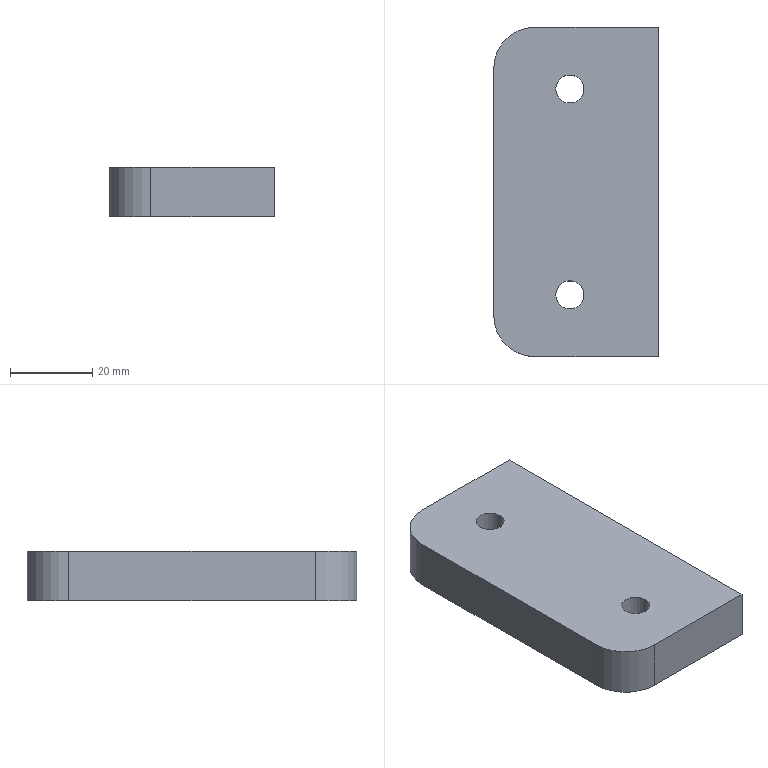Part | SolidWorks | features BaseBody 1 | 1 solid | 12 faces | box 40 x 80 x 12 mm | volume 37013 mm3 | cylinder 6 | plane 6 | commonest cylinder face diameters 6.8 x4 20 x2
STEP:
#1=CARTESIAN_POINT('',(-4.9,25.,0.));
#2=VERTEX_POINT('',#1);
#3=CARTESIAN_POINT('',(1.9,25.,0.));
#4=VERTEX_POINT('',#3);
#5=CARTESIAN_POINT('',(-1.5,25.,0.));
#6=DIRECTION('',(0.,0.,1.));
#7=DIRECTION('',(1.,0.,0.));
#8=AXIS2_PLACEMENT_3D('',#5,#6,#7);
#9=CIRCLE('',#8,3.4);
#10=EDGE_CURVE('',#2,#4,#9,.T.);
#11=ORIENTED_EDGE('',*,*,#10,.F.);
#12=CARTESIAN_POINT('',(-4.9,25.,12.));
#13=VERTEX_POINT('',#12);
#14=CARTESIAN_POINT('',(-4.9,25.,12.));
#15=DIRECTION('',(0.,0.,1.));
#16=VECTOR('',#15,1000.);
#17=LINE('',#14,#16);
#18=EDGE_CURVE('',#2,#13,#17,.T.);
#19=ORIENTED_EDGE('',*,*,#18,.T.);
#20=CARTESIAN_POINT('',(1.9,25.,12.));
#21=VERTEX_POINT('',#20);
#22=CARTESIAN_POINT('',(-1.5,25.,12.));
#23=DIRECTION('',(0.,0.,1.));
#24=DIRECTION('',(1.,0.,0.));
#25=AXIS2_PLACEMENT_3D('',#22,#23,#24);
#26=CIRCLE('',#25,3.4);
#27=EDGE_CURVE('',#13,#21,#26,.T.);
#28=ORIENTED_EDGE('',*,*,#27,.T.);
#29=CARTESIAN_POINT('',(1.9,25.,12.));
#30=DIRECTION('',(0.,0.,1.));
#31=VECTOR('',#30,1000.);
#32=LINE('',#29,#31);
#33=EDGE_CURVE('',#4,#21,#32,.T.);
#34=ORIENTED_EDGE('',*,*,#33,.F.);
#35=EDGE_LOOP('',(#11,#19,#28,#34));
#36=FACE_OUTER_BOUND('',#35,.T.);
#37=CARTESIAN_POINT('',(-1.5,25.,12.));
#38=DIRECTION('',(0.,0.,1.));
#39=DIRECTION('',(1.,0.,0.));
#40=AXIS2_PLACEMENT_3D('',#37,#38,#39);
#41=CYLINDRICAL_SURFACE('',#40,3.4);
#42=ADVANCED_FACE('',(#36),#41,.F.);
#43=CARTESIAN_POINT('',(-4.9,-25.,0.));
#44=VERTEX_POINT('',#43);
#45=CARTESIAN_POINT('',(1.9,-25.,0.));
#46=VERTEX_POINT('',#45);
#47=CARTESIAN_POINT('',(-1.5,-25.,0.));
#48=DIRECTION('',(0.,0.,1.));
#49=DIRECTION('',(1.,0.,0.));
#50=AXIS2_PLACEMENT_3D('',#47,#48,#49);
#51=CIRCLE('',#50,3.4);
#52=EDGE_CURVE('',#44,#46,#51,.T.);
#53=ORIENTED_EDGE('',*,*,#52,.F.);
#54=CARTESIAN_POINT('',(-4.9,-25.,12.));
#55=VERTEX_POINT('',#54);
#56=CARTESIAN_POINT('',(-4.9,-25.,12.));
#57=DIRECTION('',(0.,0.,1.));
#58=VECTOR('',#57,1000.);
#59=LINE('',#56,#58);
#60=EDGE_CURVE('',#44,#55,#59,.T.);
#61=ORIENTED_EDGE('',*,*,#60,.T.);
#62=CARTESIAN_POINT('',(1.9,-25.,12.));
#63=VERTEX_POINT('',#62);
#64=CARTESIAN_POINT('',(-1.5,-25.,12.));
#65=DIRECTION('',(0.,0.,1.));
#66=DIRECTION('',(1.,0.,0.));
#67=AXIS2_PLACEMENT_3D('',#64,#65,#66);
#68=CIRCLE('',#67,3.4);
#69=EDGE_CURVE('',#55,#63,#68,.T.);
#70=ORIENTED_EDGE('',*,*,#69,.T.);
#71=CARTESIAN_POINT('',(1.9,-25.,12.));
#72=DIRECTION('',(0.,0.,1.));
#73=VECTOR('',#72,1000.);
#74=LINE('',#71,#73);
#75=EDGE_CURVE('',#46,#63,#74,.T.);
#76=ORIENTED_EDGE('',*,*,#75,.F.);
#77=EDGE_LOOP('',(#53,#61,#70,#76));
#78=FACE_OUTER_BOUND('',#77,.T.);
#79=CARTESIAN_POINT('',(-1.5,-25.,12.));
#80=DIRECTION('',(0.,0.,1.));
#81=DIRECTION('',(1.,0.,0.));
#82=AXIS2_PLACEMENT_3D('',#79,#80,#81);
#83=CYLINDRICAL_SURFACE('',#82,3.4);
#84=ADVANCED_FACE('',(#78),#83,.F.);
#85=CARTESIAN_POINT('',(20.,-40.,0.));
#86=VERTEX_POINT('',#85);
#87=CARTESIAN_POINT('',(20.,40.,0.));
#88=VERTEX_POINT('',#87);
#89=CARTESIAN_POINT('',(20.,40.,0.));
#90=DIRECTION('',(0.,1.,0.));
#91=VECTOR('',#90,1000.);
#92=LINE('',#89,#91);
#93=EDGE_CURVE('',#86,#88,#92,.T.);
#94=ORIENTED_EDGE('',*,*,#93,.T.);
#95=CARTESIAN_POINT('',(20.,40.,12.));
#96=VERTEX_POINT('',#95);
#97=CARTESIAN_POINT('',(20.,40.,12.));
#98=DIRECTION('',(0.,0.,-1.));
#99=VECTOR('',#98,1000.);
#100=LINE('',#97,#99);
#101=EDGE_CURVE('',#96,#88,#100,.T.);
#102=ORIENTED_EDGE('',*,*,#101,.F.);
#103=CARTESIAN_POINT('',(20.,-40.,12.));
#104=VERTEX_POINT('',#103);
#105=CARTESIAN_POINT('',(20.,40.,12.));
#106=DIRECTION('',(0.,1.,0.));
#107=VECTOR('',#106,1000.);
#108=LINE('',#105,#107);
#109=EDGE_CURVE('',#104,#96,#108,.T.);
#110=ORIENTED_EDGE('',*,*,#109,.F.);
#111=CARTESIAN_POINT('',(20.,-40.,12.));
#112=DIRECTION('',(0.,0.,-1.));
#113=VECTOR('',#112,1000.);
#114=LINE('',#111,#113);
#115=EDGE_CURVE('',#104,#86,#114,.T.);
#116=ORIENTED_EDGE('',*,*,#115,.T.);
#117=EDGE_LOOP('',(#94,#102,#110,#116));
#118=FACE_OUTER_BOUND('',#117,.T.);
#119=CARTESIAN_POINT('',(20.,40.,12.));
#120=DIRECTION('',(-1.,0.,0.));
#121=DIRECTION('',(0.,-1.,0.));
#122=AXIS2_PLACEMENT_3D('',#119,#120,#121);
#123=PLANE('',#122);
#124=ADVANCED_FACE('',(#118),#123,.F.);
#125=CARTESIAN_POINT('',(-10.,40.,0.));
#126=VERTEX_POINT('',#125);
#127=CARTESIAN_POINT('',(-10.,40.,0.));
#128=DIRECTION('',(-1.,0.,0.));
#129=VECTOR('',#128,1000.);
#130=LINE('',#127,#129);
#131=EDGE_CURVE('',#88,#126,#130,.T.);
#132=ORIENTED_EDGE('',*,*,#131,.T.);
#133=CARTESIAN_POINT('',(-10.,40.,12.));
#134=VERTEX_POINT('',#133);
#135=CARTESIAN_POINT('',(-10.,40.,12.));
#136=DIRECTION('',(0.,0.,-1.));
#137=VECTOR('',#136,1000.);
#138=LINE('',#135,#137);
#139=EDGE_CURVE('',#134,#126,#138,.T.);
#140=ORIENTED_EDGE('',*,*,#139,.F.);
#141=CARTESIAN_POINT('',(-10.,40.,12.));
#142=DIRECTION('',(-1.,0.,0.));
#143=VECTOR('',#142,1000.);
#144=LINE('',#141,#143);
#145=EDGE_CURVE('',#96,#134,#144,.T.);
#146=ORIENTED_EDGE('',*,*,#145,.F.);
#147=ORIENTED_EDGE('',*,*,#101,.T.);
#148=EDGE_LOOP('',(#132,#140,#146,#147));
#149=FACE_OUTER_BOUND('',#148,.T.);
#150=CARTESIAN_POINT('',(-10.,40.,12.));
#151=DIRECTION('',(0.,-1.,0.));
#152=DIRECTION('',(0.,0.,-1.));
#153=AXIS2_PLACEMENT_3D('',#150,#151,#152);
#154=PLANE('',#153);
#155=ADVANCED_FACE('',(#149),#154,.F.);
#156=CARTESIAN_POINT('',(-20.,30.,0.));
#157=VERTEX_POINT('',#156);
#158=CARTESIAN_POINT('',(-10.,30.,0.));
#159=DIRECTION('',(0.,0.,1.));
#160=DIRECTION('',(1.,0.,0.));
#161=AXIS2_PLACEMENT_3D('',#158,#159,#160);
#162=CIRCLE('',#161,10.);
#163=EDGE_CURVE('',#126,#157,#162,.T.);
#164=ORIENTED_EDGE('',*,*,#163,.T.);
#165=CARTESIAN_POINT('',(-20.,30.,12.));
#166=VERTEX_POINT('',#165);
#167=CARTESIAN_POINT('',(-20.,30.,12.));
#168=DIRECTION('',(0.,0.,-1.));
#169=VECTOR('',#168,1000.);
#170=LINE('',#167,#169);
#171=EDGE_CURVE('',#166,#157,#170,.T.);
#172=ORIENTED_EDGE('',*,*,#171,.F.);
#173=CARTESIAN_POINT('',(-10.,30.,12.));
#174=DIRECTION('',(0.,0.,1.));
#175=DIRECTION('',(1.,0.,0.));
#176=AXIS2_PLACEMENT_3D('',#173,#174,#175);
#177=CIRCLE('',#176,10.);
#178=EDGE_CURVE('',#134,#166,#177,.T.);
#179=ORIENTED_EDGE('',*,*,#178,.F.);
#180=ORIENTED_EDGE('',*,*,#139,.T.);
#181=EDGE_LOOP('',(#164,#172,#179,#180));
#182=FACE_OUTER_BOUND('',#181,.T.);
#183=CARTESIAN_POINT('',(-10.,30.,12.));
#184=DIRECTION('',(0.,0.,-1.));
#185=DIRECTION('',(-1.,0.,0.));
#186=AXIS2_PLACEMENT_3D('',#183,#184,#185);
#187=CYLINDRICAL_SURFACE('',#186,10.);
#188=ADVANCED_FACE('',(#182),#187,.T.);
#189=CARTESIAN_POINT('',(-20.,-30.,0.));
#190=VERTEX_POINT('',#189);
#191=CARTESIAN_POINT('',(-20.,30.,0.));
#192=DIRECTION('',(0.,-1.,0.));
#193=VECTOR('',#192,1000.);
#194=LINE('',#191,#193);
#195=EDGE_CURVE('',#157,#190,#194,.T.);
#196=ORIENTED_EDGE('',*,*,#195,.T.);
#197=CARTESIAN_POINT('',(-20.,-30.,12.));
#198=VERTEX_POINT('',#197);
#199=CARTESIAN_POINT('',(-20.,-30.,12.));
#200=DIRECTION('',(0.,0.,-1.));
#201=VECTOR('',#200,1000.);
#202=LINE('',#199,#201);
#203=EDGE_CURVE('',#198,#190,#202,.T.);
#204=ORIENTED_EDGE('',*,*,#203,.F.);
#205=CARTESIAN_POINT('',(-20.,30.,12.));
#206=DIRECTION('',(0.,-1.,0.));
#207=VECTOR('',#206,1000.);
#208=LINE('',#205,#207);
#209=EDGE_CURVE('',#166,#198,#208,.T.);
#210=ORIENTED_EDGE('',*,*,#209,.F.);
#211=ORIENTED_EDGE('',*,*,#171,.T.);
#212=EDGE_LOOP('',(#196,#204,#210,#211));
#213=FACE_OUTER_BOUND('',#212,.T.);
#214=CARTESIAN_POINT('',(-20.,30.,12.));
#215=DIRECTION('',(1.,0.,0.));
#216=DIRECTION('',(0.,1.,0.));
#217=AXIS2_PLACEMENT_3D('',#214,#215,#216);
#218=PLANE('',#217);
#219=ADVANCED_FACE('',(#213),#218,.F.);
#220=CARTESIAN_POINT('',(-10.,-40.,0.));
#221=VERTEX_POINT('',#220);
#222=CARTESIAN_POINT('',(-10.,-30.,0.));
#223=DIRECTION('',(0.,0.,1.));
#224=DIRECTION('',(1.,0.,0.));
#225=AXIS2_PLACEMENT_3D('',#222,#223,#224);
#226=CIRCLE('',#225,10.);
#227=EDGE_CURVE('',#190,#221,#226,.T.);
#228=ORIENTED_EDGE('',*,*,#227,.T.);
#229=CARTESIAN_POINT('',(-10.,-40.,12.));
#230=VERTEX_POINT('',#229);
#231=CARTESIAN_POINT('',(-10.,-40.,12.));
#232=DIRECTION('',(0.,0.,-1.));
#233=VECTOR('',#232,1000.);
#234=LINE('',#231,#233);
#235=EDGE_CURVE('',#230,#221,#234,.T.);
#236=ORIENTED_EDGE('',*,*,#235,.F.);
#237=CARTESIAN_POINT('',(-10.,-30.,12.));
#238=DIRECTION('',(0.,0.,1.));
#239=DIRECTION('',(1.,0.,0.));
#240=AXIS2_PLACEMENT_3D('',#237,#238,#239);
#241=CIRCLE('',#240,10.);
#242=EDGE_CURVE('',#198,#230,#241,.T.);
#243=ORIENTED_EDGE('',*,*,#242,.F.);
#244=ORIENTED_EDGE('',*,*,#203,.T.);
#245=EDGE_LOOP('',(#228,#236,#243,#244));
#246=FACE_OUTER_BOUND('',#245,.T.);
#247=CARTESIAN_POINT('',(-10.,-30.,12.));
#248=DIRECTION('',(0.,0.,-1.));
#249=DIRECTION('',(-1.,0.,0.));
#250=AXIS2_PLACEMENT_3D('',#247,#248,#249);
#251=CYLINDRICAL_SURFACE('',#250,10.);
#252=ADVANCED_FACE('',(#246),#251,.T.);
#253=CARTESIAN_POINT('',(-10.,-40.,0.));
#254=DIRECTION('',(1.,0.,0.));
#255=VECTOR('',#254,1000.);
#256=LINE('',#253,#255);
#257=EDGE_CURVE('',#221,#86,#256,.T.);
#258=ORIENTED_EDGE('',*,*,#257,.T.);
#259=ORIENTED_EDGE('',*,*,#115,.F.);
#260=CARTESIAN_POINT('',(-10.,-40.,12.));
#261=DIRECTION('',(1.,0.,0.));
#262=VECTOR('',#261,1000.);
#263=LINE('',#260,#262);
#264=EDGE_CURVE('',#230,#104,#263,.T.);
#265=ORIENTED_EDGE('',*,*,#264,.F.);
#266=ORIENTED_EDGE('',*,*,#235,.T.);
#267=EDGE_LOOP('',(#258,#259,#265,#266));
#268=FACE_OUTER_BOUND('',#267,.T.);
#269=CARTESIAN_POINT('',(-10.,-40.,12.));
#270=DIRECTION('',(0.,1.,0.));
#271=DIRECTION('',(0.,0.,1.));
#272=AXIS2_PLACEMENT_3D('',#269,#270,#271);
#273=PLANE('',#272);
#274=ADVANCED_FACE('',(#268),#273,.F.);
#275=CARTESIAN_POINT('',(-1.5,25.,12.));
#276=DIRECTION('',(0.,0.,1.));
#277=DIRECTION('',(1.,0.,0.));
#278=AXIS2_PLACEMENT_3D('',#275,#276,#277);
#279=CIRCLE('',#278,3.4);
#280=EDGE_CURVE('',#21,#13,#279,.T.);
#281=ORIENTED_EDGE('',*,*,#280,.F.);
#282=ORIENTED_EDGE('',*,*,#27,.F.);
#283=EDGE_LOOP('',(#281,#282));
#284=FACE_BOUND('',#283,.T.);
#285=CARTESIAN_POINT('',(-1.5,-25.,12.));
#286=DIRECTION('',(0.,0.,1.));
#287=DIRECTION('',(1.,0.,0.));
#288=AXIS2_PLACEMENT_3D('',#285,#286,#287);
#289=CIRCLE('',#288,3.4);
#290=EDGE_CURVE('',#63,#55,#289,.T.);
#291=ORIENTED_EDGE('',*,*,#290,.F.);
#292=ORIENTED_EDGE('',*,*,#69,.F.);
#293=EDGE_LOOP('',(#291,#292));
#294=FACE_BOUND('',#293,.T.);
#295=ORIENTED_EDGE('',*,*,#109,.T.);
#296=ORIENTED_EDGE('',*,*,#145,.T.);
#297=ORIENTED_EDGE('',*,*,#178,.T.);
#298=ORIENTED_EDGE('',*,*,#209,.T.);
#299=ORIENTED_EDGE('',*,*,#242,.T.);
#300=ORIENTED_EDGE('',*,*,#264,.T.);
#301=EDGE_LOOP('',(#295,#296,#297,#298,#299,#300));
#302=FACE_OUTER_BOUND('',#301,.T.);
#303=CARTESIAN_POINT('',(-10.,-30.,12.));
#304=DIRECTION('',(0.,0.,1.));
#305=DIRECTION('',(1.,0.,0.));
#306=AXIS2_PLACEMENT_3D('',#303,#304,#305);
#307=PLANE('',#306);
#308=ADVANCED_FACE('',(#284,#294,#302),#307,.T.);
#309=CARTESIAN_POINT('',(-1.5,25.,0.));
#310=DIRECTION('',(0.,0.,1.));
#311=DIRECTION('',(1.,0.,0.));
#312=AXIS2_PLACEMENT_3D('',#309,#310,#311);
#313=CIRCLE('',#312,3.4);
#314=EDGE_CURVE('',#4,#2,#313,.T.);
#315=ORIENTED_EDGE('',*,*,#314,.T.);
#316=ORIENTED_EDGE('',*,*,#10,.T.);
#317=EDGE_LOOP('',(#315,#316));
#318=FACE_BOUND('',#317,.T.);
#319=CARTESIAN_POINT('',(-1.5,-25.,0.));
#320=DIRECTION('',(0.,0.,1.));
#321=DIRECTION('',(1.,0.,0.));
#322=AXIS2_PLACEMENT_3D('',#319,#320,#321);
#323=CIRCLE('',#322,3.4);
#324=EDGE_CURVE('',#46,#44,#323,.T.);
#325=ORIENTED_EDGE('',*,*,#324,.T.);
#326=ORIENTED_EDGE('',*,*,#52,.T.);
#327=EDGE_LOOP('',(#325,#326));
#328=FACE_BOUND('',#327,.T.);
#329=ORIENTED_EDGE('',*,*,#93,.F.);
#330=ORIENTED_EDGE('',*,*,#257,.F.);
#331=ORIENTED_EDGE('',*,*,#227,.F.);
#332=ORIENTED_EDGE('',*,*,#195,.F.);
#333=ORIENTED_EDGE('',*,*,#163,.F.);
#334=ORIENTED_EDGE('',*,*,#131,.F.);
#335=EDGE_LOOP('',(#329,#330,#331,#332,#333,#334));
#336=FACE_OUTER_BOUND('',#335,.T.);
#337=CARTESIAN_POINT('',(-10.,-30.,0.));
#338=DIRECTION('',(0.,0.,1.));
#339=DIRECTION('',(1.,0.,0.));
#340=AXIS2_PLACEMENT_3D('',#337,#338,#339);
#341=PLANE('',#340);
#342=ADVANCED_FACE('',(#318,#328,#336),#341,.F.);
#343=ORIENTED_EDGE('',*,*,#60,.F.);
#344=ORIENTED_EDGE('',*,*,#324,.F.);
#345=ORIENTED_EDGE('',*,*,#75,.T.);
#346=ORIENTED_EDGE('',*,*,#290,.T.);
#347=EDGE_LOOP('',(#343,#344,#345,#346));
#348=FACE_OUTER_BOUND('',#347,.T.);
#349=CARTESIAN_POINT('',(-1.5,-25.,12.));
#350=DIRECTION('',(0.,0.,1.));
#351=DIRECTION('',(1.,0.,0.));
#352=AXIS2_PLACEMENT_3D('',#349,#350,#351);
#353=CYLINDRICAL_SURFACE('',#352,3.4);
#354=ADVANCED_FACE('',(#348),#353,.F.);
#355=ORIENTED_EDGE('',*,*,#18,.F.);
#356=ORIENTED_EDGE('',*,*,#314,.F.);
#357=ORIENTED_EDGE('',*,*,#33,.T.);
#358=ORIENTED_EDGE('',*,*,#280,.T.);
#359=EDGE_LOOP('',(#355,#356,#357,#358));
#360=FACE_OUTER_BOUND('',#359,.T.);
#361=CARTESIAN_POINT('',(-1.5,25.,12.));
#362=DIRECTION('',(0.,0.,1.));
#363=DIRECTION('',(1.,0.,0.));
#364=AXIS2_PLACEMENT_3D('',#361,#362,#363);
#365=CYLINDRICAL_SURFACE('',#364,3.4);
#366=ADVANCED_FACE('',(#360),#365,.F.);
#367=CLOSED_SHELL('',(#42,#84,#124,#155,#188,#219,#252,#274,#308,#342,#354,#366));
#368=MANIFOLD_SOLID_BREP('',#367);
#369=CARTESIAN_POINT('',(0.,0.,0.));
#370=DIRECTION('',(0.,0.,1.));
#371=DIRECTION('',(1.,0.,0.));
#372=AXIS2_PLACEMENT_3D('',#369,#370,#371);
#373=(LENGTH_UNIT()NAMED_UNIT(*)SI_UNIT(.MILLI.,.METRE.));
#374=UNCERTAINTY_MEASURE_WITH_UNIT(LENGTH_MEASURE(0.00001),#373,'','');
#375=(NAMED_UNIT(*)PLANE_ANGLE_UNIT()SI_UNIT($,.RADIAN.));
#376=(NAMED_UNIT(*)SI_UNIT($,.STERADIAN.)SOLID_ANGLE_UNIT());
#377=(GEOMETRIC_REPRESENTATION_CONTEXT(3)GLOBAL_UNCERTAINTY_ASSIGNED_CONTEXT((#374))GLOBAL_UNIT_ASSIGNED_CONTEXT((#373,#375,#376))REPRESENTATION_CONTEXT('',''));
#378=ADVANCED_BREP_SHAPE_REPRESENTATION('',(#368,#372),#377);